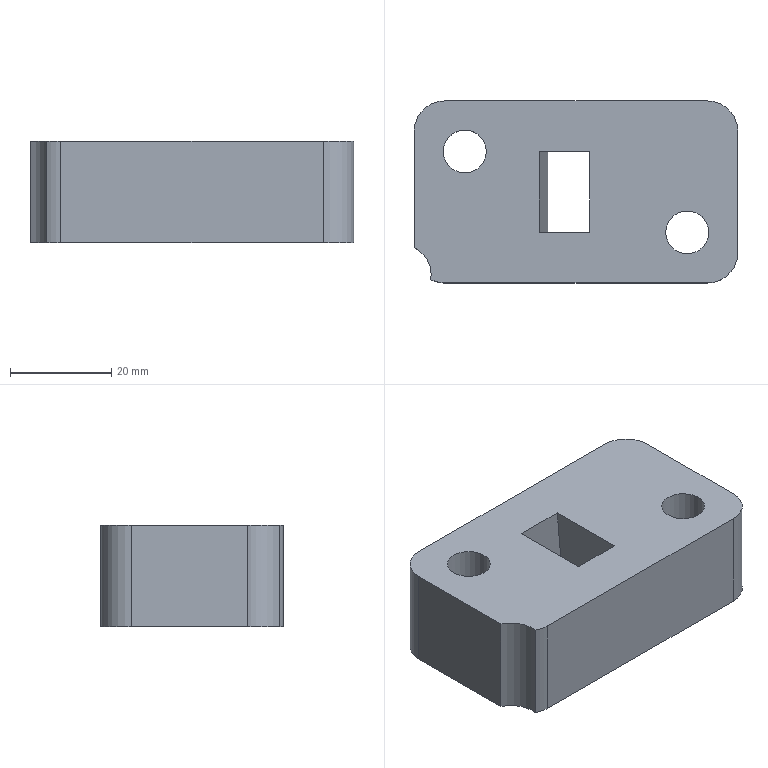Part | STEP file | solid 105 | 1 solid | 29 faces | box 64 x 36 x 20 mm | volume 38008 mm3 | plane 18 | cylinder 9 | other 2 | commonest cylinder face diameters 12 x5 8.5 x2 14 x2